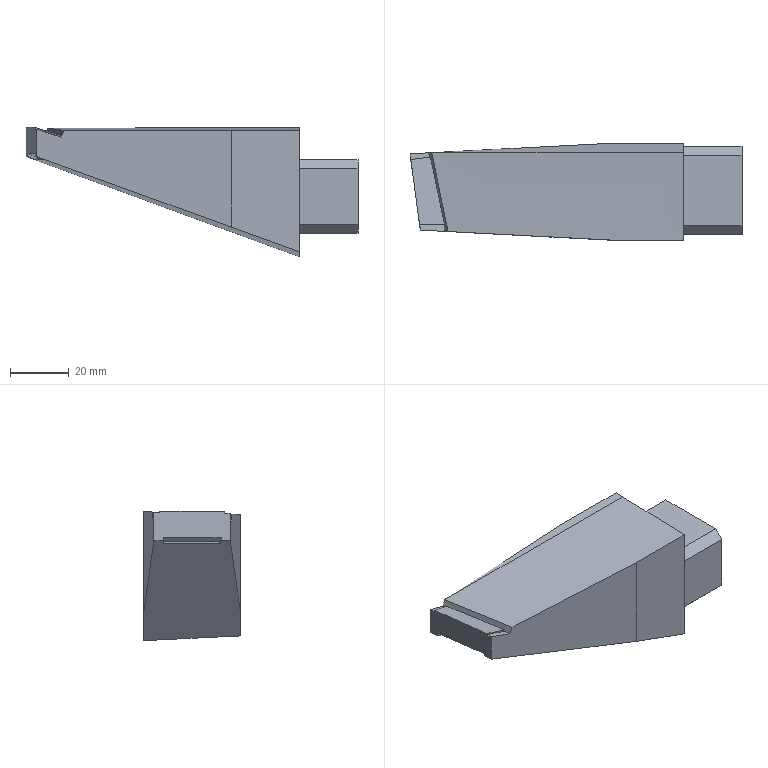Part | STEP file | P011002S002-001 | 1 solid | 63 faces | box 113.158 x 33 x 44.092 mm | volume 87912 mm3 | plane 35 | other 10 | spline 8 | cone 7 | cylinder 3 | commonest cylinder face diameters 6.8 x1 7.973 x1 8 x1